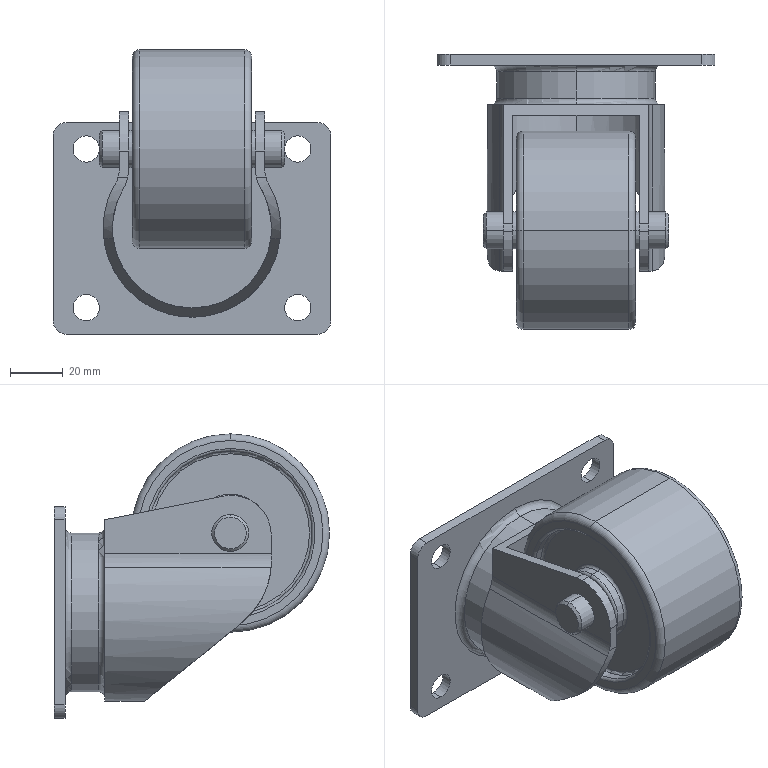Part | SolidWorks | features ICE 10, Fillet 8, Chamfer 1, Extrusion 1 | 1 solid | 97 faces | box 105 x 104 x 107.5 mm | volume 293798 mm3 | cylinder 45 | torus 24 | plane 24 | cone 4 | commonest cylinder face diameters 10 x12 14 x8 27.5 x4 30 x4 60 x4 62 x4